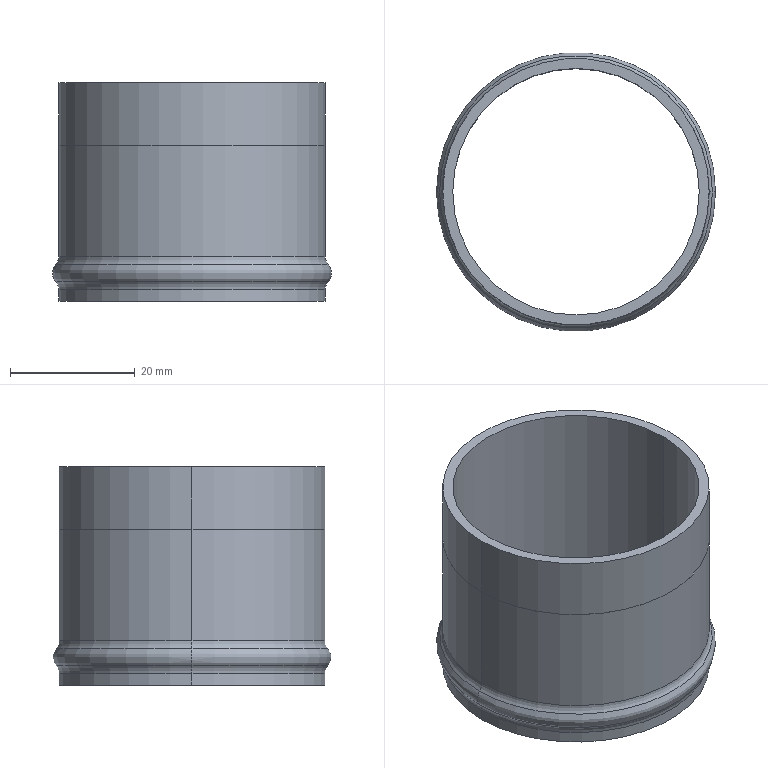Part | SolidWorks | features ICE 1, RevolutionThin 1 | 1 solid | 25 faces | box 44.7 x 44.7 x 35 mm | volume 7344 mm3 | torus 12 | cylinder 10 | plane 3 | commonest cylinder face diameters 39.5 x4 42.7 x4 42.68 x2
STEP:
#1=CARTESIAN_POINT('',(21.34,0.,-10.));
#2=VERTEX_POINT('',#1);
#3=CARTESIAN_POINT('',(-21.34,0.,-10.));
#4=VERTEX_POINT('',#3);
#5=CARTESIAN_POINT('',(0.,0.,-10.));
#6=DIRECTION('',(0.,0.,1.));
#7=DIRECTION('',(1.,0.,0.));
#8=AXIS2_PLACEMENT_3D('',#5,#6,#7);
#9=CIRCLE('',#8,21.34);
#10=EDGE_CURVE('',#2,#4,#9,.T.);
#11=ORIENTED_EDGE('',*,*,#10,.T.);
#12=CARTESIAN_POINT('',(-21.34,0.,0.));
#13=VERTEX_POINT('',#12);
#14=CARTESIAN_POINT('',(-21.34,0.,-10.));
#15=DIRECTION('',(0.,0.,1.));
#16=VECTOR('',#15,1000.);
#17=LINE('',#14,#16);
#18=EDGE_CURVE('',#4,#13,#17,.T.);
#19=ORIENTED_EDGE('',*,*,#18,.T.);
#20=CARTESIAN_POINT('',(21.34,0.,0.));
#21=VERTEX_POINT('',#20);
#22=CARTESIAN_POINT('',(0.,0.,0.));
#23=DIRECTION('',(0.,0.,1.));
#24=DIRECTION('',(1.,0.,0.));
#25=AXIS2_PLACEMENT_3D('',#22,#23,#24);
#26=CIRCLE('',#25,21.34);
#27=EDGE_CURVE('',#21,#13,#26,.T.);
#28=ORIENTED_EDGE('',*,*,#27,.F.);
#29=CARTESIAN_POINT('',(21.34,0.,-10.));
#30=DIRECTION('',(0.,0.,1.));
#31=VECTOR('',#30,1000.);
#32=LINE('',#29,#31);
#33=EDGE_CURVE('',#2,#21,#32,.T.);
#34=ORIENTED_EDGE('',*,*,#33,.F.);
#35=EDGE_LOOP('',(#11,#19,#28,#34));
#36=FACE_OUTER_BOUND('',#35,.T.);
#37=CARTESIAN_POINT('',(0.,0.,-10.));
#38=DIRECTION('',(0.,0.,1.));
#39=DIRECTION('',(1.,0.,0.));
#40=AXIS2_PLACEMENT_3D('',#37,#38,#39);
#41=CYLINDRICAL_SURFACE('',#40,21.34);
#42=ADVANCED_FACE('',(#36),#41,.T.);
#43=CARTESIAN_POINT('',(20.65,0.,-30.765));
#44=VERTEX_POINT('',#43);
#45=CARTESIAN_POINT('',(-20.65,0.,-30.765));
#46=VERTEX_POINT('',#45);
#47=CARTESIAN_POINT('',(0.,0.,-30.765));
#48=DIRECTION('',(0.,0.,1.));
#49=DIRECTION('',(1.,0.,0.));
#50=AXIS2_PLACEMENT_3D('',#47,#48,#49);
#51=CIRCLE('',#50,20.65);
#52=EDGE_CURVE('',#44,#46,#51,.T.);
#53=ORIENTED_EDGE('',*,*,#52,.T.);
#54=CARTESIAN_POINT('',(-19.75,0.,-33.146));
#55=VERTEX_POINT('',#54);
#56=CARTESIAN_POINT('',(-23.35,0.,-33.146));
#57=DIRECTION('',(0.,1.,0.));
#58=DIRECTION('',(-1.,0.,0.));
#59=AXIS2_PLACEMENT_3D('',#56,#57,#58);
#60=CIRCLE('',#59,3.6);
#61=EDGE_CURVE('',#46,#55,#60,.T.);
#62=ORIENTED_EDGE('',*,*,#61,.T.);
#63=CARTESIAN_POINT('',(19.75,0.,-33.146));
#64=VERTEX_POINT('',#63);
#65=CARTESIAN_POINT('',(0.,0.,-33.146));
#66=DIRECTION('',(0.,0.,1.));
#67=DIRECTION('',(1.,0.,0.));
#68=AXIS2_PLACEMENT_3D('',#65,#66,#67);
#69=CIRCLE('',#68,19.75);
#70=EDGE_CURVE('',#64,#55,#69,.T.);
#71=ORIENTED_EDGE('',*,*,#70,.F.);
#72=CARTESIAN_POINT('',(23.35,0.,-33.146));
#73=DIRECTION('',(0.,-1.,0.));
#74=DIRECTION('',(0.,0.,-1.));
#75=AXIS2_PLACEMENT_3D('',#72,#73,#74);
#76=CIRCLE('',#75,3.6);
#77=EDGE_CURVE('',#44,#64,#76,.T.);
#78=ORIENTED_EDGE('',*,*,#77,.F.);
#79=EDGE_LOOP('',(#53,#62,#71,#78));
#80=FACE_OUTER_BOUND('',#79,.T.);
#81=CARTESIAN_POINT('',(0.,0.,-33.146));
#82=DIRECTION('',(0.,0.,1.));
#83=DIRECTION('',(1.,0.,0.));
#84=AXIS2_PLACEMENT_3D('',#81,#82,#83);
#85=TOROIDAL_SURFACE('',#84,23.35,3.6);
#86=ADVANCED_FACE('',(#80),#85,.T.);
#87=CARTESIAN_POINT('',(0.,0.,-30.765));
#88=DIRECTION('',(0.,0.,1.));
#89=DIRECTION('',(1.,0.,0.));
#90=AXIS2_PLACEMENT_3D('',#87,#88,#89);
#91=CIRCLE('',#90,20.65);
#92=EDGE_CURVE('',#46,#44,#91,.T.);
#93=ORIENTED_EDGE('',*,*,#92,.F.);
#94=CARTESIAN_POINT('',(-20.65,0.,-30.235));
#95=VERTEX_POINT('',#94);
#96=CARTESIAN_POINT('',(-20.35,0.,-30.5));
#97=DIRECTION('',(0.,1.,0.));
#98=DIRECTION('',(-1.,0.,0.));
#99=AXIS2_PLACEMENT_3D('',#96,#97,#98);
#100=CIRCLE('',#99,0.4);
#101=EDGE_CURVE('',#46,#95,#100,.T.);
#102=ORIENTED_EDGE('',*,*,#101,.T.);
#103=CARTESIAN_POINT('',(20.65,0.,-30.235));
#104=VERTEX_POINT('',#103);
#105=CARTESIAN_POINT('',(0.,0.,-30.235));
#106=DIRECTION('',(0.,0.,1.));
#107=DIRECTION('',(1.,0.,0.));
#108=AXIS2_PLACEMENT_3D('',#105,#106,#107);
#109=CIRCLE('',#108,20.65);
#110=EDGE_CURVE('',#95,#104,#109,.T.);
#111=ORIENTED_EDGE('',*,*,#110,.T.);
#112=CARTESIAN_POINT('',(20.35,0.,-30.5));
#113=DIRECTION('',(0.,-1.,0.));
#114=DIRECTION('',(0.,0.,-1.));
#115=AXIS2_PLACEMENT_3D('',#112,#113,#114);
#116=CIRCLE('',#115,0.4);
#117=EDGE_CURVE('',#44,#104,#116,.T.);
#118=ORIENTED_EDGE('',*,*,#117,.F.);
#119=EDGE_LOOP('',(#93,#102,#111,#118));
#120=FACE_OUTER_BOUND('',#119,.T.);
#121=CARTESIAN_POINT('',(0.,0.,-30.5));
#122=DIRECTION('',(0.,0.,1.));
#123=DIRECTION('',(1.,0.,0.));
#124=AXIS2_PLACEMENT_3D('',#121,#122,#123);
#125=TOROIDAL_SURFACE('',#124,20.35,0.4);
#126=ADVANCED_FACE('',(#120),#125,.F.);
#127=CARTESIAN_POINT('',(19.75,0.,-27.854));
#128=VERTEX_POINT('',#127);
#129=CARTESIAN_POINT('',(-19.75,0.,-27.854));
#130=VERTEX_POINT('',#129);
#131=CARTESIAN_POINT('',(0.,0.,-27.854));
#132=DIRECTION('',(0.,0.,1.));
#133=DIRECTION('',(1.,0.,0.));
#134=AXIS2_PLACEMENT_3D('',#131,#132,#133);
#135=CIRCLE('',#134,19.75);
#136=EDGE_CURVE('',#128,#130,#135,.T.);
#137=ORIENTED_EDGE('',*,*,#136,.T.);
#138=CARTESIAN_POINT('',(-23.35,0.,-27.854));
#139=DIRECTION('',(0.,1.,0.));
#140=DIRECTION('',(-1.,0.,0.));
#141=AXIS2_PLACEMENT_3D('',#138,#139,#140);
#142=CIRCLE('',#141,3.6);
#143=EDGE_CURVE('',#130,#95,#142,.T.);
#144=ORIENTED_EDGE('',*,*,#143,.T.);
#145=CARTESIAN_POINT('',(0.,0.,-30.235));
#146=DIRECTION('',(0.,0.,1.));
#147=DIRECTION('',(1.,0.,0.));
#148=AXIS2_PLACEMENT_3D('',#145,#146,#147);
#149=CIRCLE('',#148,20.65);
#150=EDGE_CURVE('',#104,#95,#149,.T.);
#151=ORIENTED_EDGE('',*,*,#150,.F.);
#152=CARTESIAN_POINT('',(23.35,0.,-27.854));
#153=DIRECTION('',(0.,-1.,0.));
#154=DIRECTION('',(0.,0.,-1.));
#155=AXIS2_PLACEMENT_3D('',#152,#153,#154);
#156=CIRCLE('',#155,3.6);
#157=EDGE_CURVE('',#128,#104,#156,.T.);
#158=ORIENTED_EDGE('',*,*,#157,.F.);
#159=EDGE_LOOP('',(#137,#144,#151,#158));
#160=FACE_OUTER_BOUND('',#159,.T.);
#161=CARTESIAN_POINT('',(0.,0.,-27.854));
#162=DIRECTION('',(0.,0.,1.));
#163=DIRECTION('',(1.,0.,0.));
#164=AXIS2_PLACEMENT_3D('',#161,#162,#163);
#165=TOROIDAL_SURFACE('',#164,23.35,3.6);
#166=ADVANCED_FACE('',(#160),#165,.T.);
#167=CARTESIAN_POINT('',(0.,0.,-27.854));
#168=DIRECTION('',(0.,0.,1.));
#169=DIRECTION('',(1.,0.,0.));
#170=AXIS2_PLACEMENT_3D('',#167,#168,#169);
#171=CIRCLE('',#170,19.75);
#172=EDGE_CURVE('',#130,#128,#171,.T.);
#173=ORIENTED_EDGE('',*,*,#172,.F.);
#174=CARTESIAN_POINT('',(-19.75,0.,0.));
#175=VERTEX_POINT('',#174);
#176=CARTESIAN_POINT('',(-19.75,0.,0.));
#177=DIRECTION('',(0.,0.,1.));
#178=VECTOR('',#177,1000.);
#179=LINE('',#176,#178);
#180=EDGE_CURVE('',#130,#175,#179,.T.);
#181=ORIENTED_EDGE('',*,*,#180,.T.);
#182=CARTESIAN_POINT('',(19.75,0.,0.));
#183=VERTEX_POINT('',#182);
#184=CARTESIAN_POINT('',(0.,0.,0.));
#185=DIRECTION('',(0.,0.,1.));
#186=DIRECTION('',(1.,0.,0.));
#187=AXIS2_PLACEMENT_3D('',#184,#185,#186);
#188=CIRCLE('',#187,19.75);
#189=EDGE_CURVE('',#175,#183,#188,.T.);
#190=ORIENTED_EDGE('',*,*,#189,.T.);
#191=CARTESIAN_POINT('',(19.75,0.,0.));
#192=DIRECTION('',(0.,0.,1.));
#193=VECTOR('',#192,1000.);
#194=LINE('',#191,#193);
#195=EDGE_CURVE('',#128,#183,#194,.T.);
#196=ORIENTED_EDGE('',*,*,#195,.F.);
#197=EDGE_LOOP('',(#173,#181,#190,#196));
#198=FACE_OUTER_BOUND('',#197,.T.);
#199=CARTESIAN_POINT('',(0.,0.,0.));
#200=DIRECTION('',(0.,0.,1.));
#201=DIRECTION('',(1.,0.,0.));
#202=AXIS2_PLACEMENT_3D('',#199,#200,#201);
#203=CYLINDRICAL_SURFACE('',#202,19.75);
#204=ADVANCED_FACE('',(#198),#203,.F.);
#205=CARTESIAN_POINT('',(-21.35,0.,-27.854));
#206=VERTEX_POINT('',#205);
#207=CARTESIAN_POINT('',(21.35,0.,-27.854));
#208=VERTEX_POINT('',#207);
#209=CARTESIAN_POINT('',(0.,0.,-27.854));
#210=DIRECTION('',(0.,0.,1.));
#211=DIRECTION('',(1.,0.,0.));
#212=AXIS2_PLACEMENT_3D('',#209,#210,#211);
#213=CIRCLE('',#212,21.35);
#214=EDGE_CURVE('',#206,#208,#213,.T.);
#215=ORIENTED_EDGE('',*,*,#214,.F.);
#216=CARTESIAN_POINT('',(-21.85,0.,-29.177));
#217=VERTEX_POINT('',#216);
#218=CARTESIAN_POINT('',(-23.35,0.,-27.854));
#219=DIRECTION('',(0.,1.,0.));
#220=DIRECTION('',(-1.,0.,0.));
#221=AXIS2_PLACEMENT_3D('',#218,#219,#220);
#222=CIRCLE('',#221,2.);
#223=EDGE_CURVE('',#206,#217,#222,.T.);
#224=ORIENTED_EDGE('',*,*,#223,.T.);
#225=CARTESIAN_POINT('',(21.85,0.,-29.177));
#226=VERTEX_POINT('',#225);
#227=CARTESIAN_POINT('',(0.,0.,-29.177));
#228=DIRECTION('',(0.,0.,1.));
#229=DIRECTION('',(1.,0.,0.));
#230=AXIS2_PLACEMENT_3D('',#227,#228,#229);
#231=CIRCLE('',#230,21.85);
#232=EDGE_CURVE('',#217,#226,#231,.T.);
#233=ORIENTED_EDGE('',*,*,#232,.T.);
#234=CARTESIAN_POINT('',(23.35,0.,-27.854));
#235=DIRECTION('',(0.,-1.,0.));
#236=DIRECTION('',(0.,0.,-1.));
#237=AXIS2_PLACEMENT_3D('',#234,#235,#236);
#238=CIRCLE('',#237,2.);
#239=EDGE_CURVE('',#208,#226,#238,.T.);
#240=ORIENTED_EDGE('',*,*,#239,.F.);
#241=EDGE_LOOP('',(#215,#224,#233,#240));
#242=FACE_OUTER_BOUND('',#241,.T.);
#243=CARTESIAN_POINT('',(0.,0.,-27.854));
#244=DIRECTION('',(0.,0.,1.));
#245=DIRECTION('',(1.,0.,0.));
#246=AXIS2_PLACEMENT_3D('',#243,#244,#245);
#247=TOROIDAL_SURFACE('',#246,23.35,2.);
#248=ADVANCED_FACE('',(#242),#247,.F.);
#249=CARTESIAN_POINT('',(21.85,0.,-31.823));
#250=VERTEX_POINT('',#249);
#251=CARTESIAN_POINT('',(-21.85,0.,-31.823));
#252=VERTEX_POINT('',#251);
#253=CARTESIAN_POINT('',(0.,0.,-31.823));
#254=DIRECTION('',(0.,0.,1.));
#255=DIRECTION('',(1.,0.,0.));
#256=AXIS2_PLACEMENT_3D('',#253,#254,#255);
#257=CIRCLE('',#256,21.85);
#258=EDGE_CURVE('',#250,#252,#257,.T.);
#259=ORIENTED_EDGE('',*,*,#258,.T.);
#260=CARTESIAN_POINT('',(-20.35,0.,-30.5));
#261=DIRECTION('',(0.,1.,0.));
#262=DIRECTION('',(-1.,0.,0.));
#263=AXIS2_PLACEMENT_3D('',#260,#261,#262);
#264=CIRCLE('',#263,2.);
#265=EDGE_CURVE('',#252,#217,#264,.T.);
#266=ORIENTED_EDGE('',*,*,#265,.T.);
#267=CARTESIAN_POINT('',(0.,0.,-29.177));
#268=DIRECTION('',(0.,0.,1.));
#269=DIRECTION('',(1.,0.,0.));
#270=AXIS2_PLACEMENT_3D('',#267,#268,#269);
#271=CIRCLE('',#270,21.85);
#272=EDGE_CURVE('',#226,#217,#271,.T.);
#273=ORIENTED_EDGE('',*,*,#272,.F.);
#274=CARTESIAN_POINT('',(20.35,0.,-30.5));
#275=DIRECTION('',(0.,-1.,0.));
#276=DIRECTION('',(0.,0.,-1.));
#277=AXIS2_PLACEMENT_3D('',#274,#275,#276);
#278=CIRCLE('',#277,2.);
#279=EDGE_CURVE('',#250,#226,#278,.T.);
#280=ORIENTED_EDGE('',*,*,#279,.F.);
#281=EDGE_LOOP('',(#259,#266,#273,#280));
#282=FACE_OUTER_BOUND('',#281,.T.);
#283=CARTESIAN_POINT('',(0.,0.,-30.5));
#284=DIRECTION('',(0.,0.,1.));
#285=DIRECTION('',(1.,0.,0.));
#286=AXIS2_PLACEMENT_3D('',#283,#284,#285);
#287=TOROIDAL_SURFACE('',#286,20.35,2.);
#288=ADVANCED_FACE('',(#282),#287,.T.);
#289=CARTESIAN_POINT('',(0.,0.,-31.823));
#290=DIRECTION('',(0.,0.,1.));
#291=DIRECTION('',(1.,0.,0.));
#292=AXIS2_PLACEMENT_3D('',#289,#290,#291);
#293=CIRCLE('',#292,21.85);
#294=EDGE_CURVE('',#252,#250,#293,.T.);
#295=ORIENTED_EDGE('',*,*,#294,.F.);
#296=CARTESIAN_POINT('',(-21.35,0.,-33.146));
#297=VERTEX_POINT('',#296);
#298=CARTESIAN_POINT('',(-23.35,0.,-33.146));
#299=DIRECTION('',(0.,1.,0.));
#300=DIRECTION('',(-1.,0.,0.));
#301=AXIS2_PLACEMENT_3D('',#298,#299,#300);
#302=CIRCLE('',#301,2.);
#303=EDGE_CURVE('',#252,#297,#302,.T.);
#304=ORIENTED_EDGE('',*,*,#303,.T.);
#305=CARTESIAN_POINT('',(21.35,0.,-33.146));
#306=VERTEX_POINT('',#305);
#307=CARTESIAN_POINT('',(0.,0.,-33.146));
#308=DIRECTION('',(0.,0.,1.));
#309=DIRECTION('',(1.,0.,0.));
#310=AXIS2_PLACEMENT_3D('',#307,#308,#309);
#311=CIRCLE('',#310,21.35);
#312=EDGE_CURVE('',#297,#306,#311,.T.);
#313=ORIENTED_EDGE('',*,*,#312,.T.);
#314=CARTESIAN_POINT('',(23.35,0.,-33.146));
#315=DIRECTION('',(0.,-1.,0.));
#316=DIRECTION('',(0.,0.,-1.));
#317=AXIS2_PLACEMENT_3D('',#314,#315,#316);
#318=CIRCLE('',#317,2.);
#319=EDGE_CURVE('',#250,#306,#318,.T.);
#320=ORIENTED_EDGE('',*,*,#319,.F.);
#321=EDGE_LOOP('',(#295,#304,#313,#320));
#322=FACE_OUTER_BOUND('',#321,.T.);
#323=CARTESIAN_POINT('',(0.,0.,-33.146));
#324=DIRECTION('',(0.,0.,1.));
#325=DIRECTION('',(1.,0.,0.));
#326=AXIS2_PLACEMENT_3D('',#323,#324,#325);
#327=TOROIDAL_SURFACE('',#326,23.35,2.);
#328=ADVANCED_FACE('',(#322),#327,.F.);
#329=CARTESIAN_POINT('',(21.35,0.,-35.));
#330=VERTEX_POINT('',#329);
#331=CARTESIAN_POINT('',(-21.35,0.,-35.));
#332=VERTEX_POINT('',#331);
#333=CARTESIAN_POINT('',(0.,0.,-35.));
#334=DIRECTION('',(0.,0.,1.));
#335=DIRECTION('',(1.,0.,0.));
#336=AXIS2_PLACEMENT_3D('',#333,#334,#335);
#337=CIRCLE('',#336,21.35);
#338=EDGE_CURVE('',#330,#332,#337,.T.);
#339=ORIENTED_EDGE('',*,*,#338,.T.);
#340=CARTESIAN_POINT('',(-21.35,0.,0.));
#341=DIRECTION('',(0.,0.,1.));
#342=VECTOR('',#341,1000.);
#343=LINE('',#340,#342);
#344=EDGE_CURVE('',#332,#297,#343,.T.);
#345=ORIENTED_EDGE('',*,*,#344,.T.);
#346=CARTESIAN_POINT('',(0.,0.,-33.146));
#347=DIRECTION('',(0.,0.,1.));
#348=DIRECTION('',(1.,0.,0.));
#349=AXIS2_PLACEMENT_3D('',#346,#347,#348);
#350=CIRCLE('',#349,21.35);
#351=EDGE_CURVE('',#306,#297,#350,.T.);
#352=ORIENTED_EDGE('',*,*,#351,.F.);
#353=CARTESIAN_POINT('',(21.35,0.,0.));
#354=DIRECTION('',(0.,0.,1.));
#355=VECTOR('',#354,1000.);
#356=LINE('',#353,#355);
#357=EDGE_CURVE('',#330,#306,#356,.T.);
#358=ORIENTED_EDGE('',*,*,#357,.F.);
#359=EDGE_LOOP('',(#339,#345,#352,#358));
#360=FACE_OUTER_BOUND('',#359,.T.);
#361=CARTESIAN_POINT('',(0.,0.,0.));
#362=DIRECTION('',(0.,0.,1.));
#363=DIRECTION('',(1.,0.,0.));
#364=AXIS2_PLACEMENT_3D('',#361,#362,#363);
#365=CYLINDRICAL_SURFACE('',#364,21.35);
#366=ADVANCED_FACE('',(#360),#365,.T.);
#367=CARTESIAN_POINT('',(-19.75,0.,-35.));
#368=VERTEX_POINT('',#367);
#369=CARTESIAN_POINT('',(19.75,0.,-35.));
#370=VERTEX_POINT('',#369);
#371=CARTESIAN_POINT('',(0.,0.,-35.));
#372=DIRECTION('',(0.,0.,1.));
#373=DIRECTION('',(1.,0.,0.));
#374=AXIS2_PLACEMENT_3D('',#371,#372,#373);
#375=CIRCLE('',#374,19.75);
#376=EDGE_CURVE('',#368,#370,#375,.T.);
#377=ORIENTED_EDGE('',*,*,#376,.F.);
#378=CARTESIAN_POINT('',(-19.75,0.,0.));
#379=DIRECTION('',(0.,0.,1.));
#380=VECTOR('',#379,1000.);
#381=LINE('',#378,#380);
#382=EDGE_CURVE('',#368,#55,#381,.T.);
#383=ORIENTED_EDGE('',*,*,#382,.T.);
#384=CARTESIAN_POINT('',(0.,0.,-33.146));
#385=DIRECTION('',(0.,0.,1.));
#386=DIRECTION('',(1.,0.,0.));
#387=AXIS2_PLACEMENT_3D('',#384,#385,#386);
#388=CIRCLE('',#387,19.75);
#389=EDGE_CURVE('',#55,#64,#388,.T.);
#390=ORIENTED_EDGE('',*,*,#389,.T.);
#391=CARTESIAN_POINT('',(19.75,0.,0.));
#392=DIRECTION('',(0.,0.,1.));
#393=VECTOR('',#392,1000.);
#394=LINE('',#391,#393);
#395=EDGE_CURVE('',#370,#64,#394,.T.);
#396=ORIENTED_EDGE('',*,*,#395,.F.);
#397=EDGE_LOOP('',(#377,#383,#390,#396));
#398=FACE_OUTER_BOUND('',#397,.T.);
#399=CARTESIAN_POINT('',(0.,0.,0.));
#400=DIRECTION('',(0.,0.,1.));
#401=DIRECTION('',(1.,0.,0.));
#402=AXIS2_PLACEMENT_3D('',#399,#400,#401);
#403=CYLINDRICAL_SURFACE('',#402,19.75);
#404=ADVANCED_FACE('',(#398),#403,.F.);
#405=CARTESIAN_POINT('',(0.,0.,-27.854));
#406=DIRECTION('',(0.,0.,1.));
#407=DIRECTION('',(1.,0.,0.));
#408=AXIS2_PLACEMENT_3D('',#405,#406,#407);
#409=CIRCLE('',#408,21.35);
#410=EDGE_CURVE('',#208,#206,#409,.T.);
#411=ORIENTED_EDGE('',*,*,#410,.T.);
#412=CARTESIAN_POINT('',(-21.35,0.,-10.));
#413=VERTEX_POINT('',#412);
#414=CARTESIAN_POINT('',(-21.35,0.,0.));
#415=DIRECTION('',(0.,0.,1.));
#416=VECTOR('',#415,1000.);
#417=LINE('',#414,#416);
#418=EDGE_CURVE('',#206,#413,#417,.T.);
#419=ORIENTED_EDGE('',*,*,#418,.T.);
#420=CARTESIAN_POINT('',(21.35,0.,-10.));
#421=VERTEX_POINT('',#420);
#422=CARTESIAN_POINT('',(0.,0.,-10.));
#423=DIRECTION('',(0.,0.,1.));
#424=DIRECTION('',(1.,0.,0.));
#425=AXIS2_PLACEMENT_3D('',#422,#423,#424);
#426=CIRCLE('',#425,21.35);
#427=EDGE_CURVE('',#421,#413,#426,.T.);
#428=ORIENTED_EDGE('',*,*,#427,.F.);
#429=CARTESIAN_POINT('',(21.35,0.,0.));
#430=DIRECTION('',(0.,0.,1.));
#431=VECTOR('',#430,1000.);
#432=LINE('',#429,#431);
#433=EDGE_CURVE('',#208,#421,#432,.T.);
#434=ORIENTED_EDGE('',*,*,#433,.F.);
#435=EDGE_LOOP('',(#411,#419,#428,#434));
#436=FACE_OUTER_BOUND('',#435,.T.);
#437=CARTESIAN_POINT('',(0.,0.,0.));
#438=DIRECTION('',(0.,0.,1.));
#439=DIRECTION('',(1.,0.,0.));
#440=AXIS2_PLACEMENT_3D('',#437,#438,#439);
#441=CYLINDRICAL_SURFACE('',#440,21.35);
#442=ADVANCED_FACE('',(#436),#441,.T.);
#443=ORIENTED_EDGE('',*,*,#418,.F.);
#444=ORIENTED_EDGE('',*,*,#214,.T.);
#445=ORIENTED_EDGE('',*,*,#433,.T.);
#446=CARTESIAN_POINT('',(0.,0.,-10.));
#447=DIRECTION('',(0.,0.,1.));
#448=DIRECTION('',(1.,0.,0.));
#449=AXIS2_PLACEMENT_3D('',#446,#447,#448);
#450=CIRCLE('',#449,21.35);
#451=EDGE_CURVE('',#413,#421,#450,.T.);
#452=ORIENTED_EDGE('',*,*,#451,.F.);
#453=EDGE_LOOP('',(#443,#444,#445,#452));
#454=FACE_OUTER_BOUND('',#453,.T.);
#455=CARTESIAN_POINT('',(0.,0.,0.));
#456=DIRECTION('',(0.,0.,1.));
#457=DIRECTION('',(1.,0.,0.));
#458=AXIS2_PLACEMENT_3D('',#455,#456,#457);
#459=CYLINDRICAL_SURFACE('',#458,21.35);
#460=ADVANCED_FACE('',(#454),#459,.T.);
#461=CARTESIAN_POINT('',(0.,0.,0.));
#462=DIRECTION('',(0.,0.,1.));
#463=DIRECTION('',(1.,0.,0.));
#464=AXIS2_PLACEMENT_3D('',#461,#462,#463);
#465=CIRCLE('',#464,19.75);
#466=EDGE_CURVE('',#183,#175,#465,.T.);
#467=ORIENTED_EDGE('',*,*,#466,.F.);
#468=ORIENTED_EDGE('',*,*,#189,.F.);
#469=EDGE_LOOP('',(#467,#468));
#470=FACE_BOUND('',#469,.T.);
#471=ORIENTED_EDGE('',*,*,#27,.T.);
#472=CARTESIAN_POINT('',(0.,0.,0.));
#473=DIRECTION('',(0.,0.,1.));
#474=DIRECTION('',(1.,0.,0.));
#475=AXIS2_PLACEMENT_3D('',#472,#473,#474);
#476=CIRCLE('',#475,21.34);
#477=EDGE_CURVE('',#13,#21,#476,.T.);
#478=ORIENTED_EDGE('',*,*,#477,.T.);
#479=EDGE_LOOP('',(#471,#478));
#480=FACE_OUTER_BOUND('',#479,.T.);
#481=CARTESIAN_POINT('',(0.,19.75,0.));
#482=DIRECTION('',(0.,0.,1.));
#483=DIRECTION('',(1.,0.,0.));
#484=AXIS2_PLACEMENT_3D('',#481,#482,#483);
#485=PLANE('',#484);
#486=ADVANCED_FACE('',(#470,#480),#485,.T.);
#487=ORIENTED_EDGE('',*,*,#382,.F.);
#488=CARTESIAN_POINT('',(0.,0.,-35.));
#489=DIRECTION('',(0.,0.,1.));
#490=DIRECTION('',(1.,0.,0.));
#491=AXIS2_PLACEMENT_3D('',#488,#489,#490);
#492=CIRCLE('',#491,19.75);
#493=EDGE_CURVE('',#370,#368,#492,.T.);
#494=ORIENTED_EDGE('',*,*,#493,.F.);
#495=ORIENTED_EDGE('',*,*,#395,.T.);
#496=ORIENTED_EDGE('',*,*,#70,.T.);
#497=EDGE_LOOP('',(#487,#494,#495,#496));
#498=FACE_OUTER_BOUND('',#497,.T.);
#499=CARTESIAN_POINT('',(0.,0.,0.));
#500=DIRECTION('',(0.,0.,1.));
#501=DIRECTION('',(1.,0.,0.));
#502=AXIS2_PLACEMENT_3D('',#499,#500,#501);
#503=CYLINDRICAL_SURFACE('',#502,19.75);
#504=ADVANCED_FACE('',(#498),#503,.F.);
#505=ORIENTED_EDGE('',*,*,#493,.T.);
#506=ORIENTED_EDGE('',*,*,#376,.T.);
#507=EDGE_LOOP('',(#505,#506));
#508=FACE_BOUND('',#507,.T.);
#509=ORIENTED_EDGE('',*,*,#338,.F.);
#510=CARTESIAN_POINT('',(0.,0.,-35.));
#511=DIRECTION('',(0.,0.,1.));
#512=DIRECTION('',(1.,0.,0.));
#513=AXIS2_PLACEMENT_3D('',#510,#511,#512);
#514=CIRCLE('',#513,21.35);
#515=EDGE_CURVE('',#332,#330,#514,.T.);
#516=ORIENTED_EDGE('',*,*,#515,.F.);
#517=EDGE_LOOP('',(#509,#516));
#518=FACE_OUTER_BOUND('',#517,.T.);
#519=CARTESIAN_POINT('',(0.,21.35,-35.));
#520=DIRECTION('',(0.,0.,-1.));
#521=DIRECTION('',(-1.,0.,0.));
#522=AXIS2_PLACEMENT_3D('',#519,#520,#521);
#523=PLANE('',#522);
#524=ADVANCED_FACE('',(#508,#518),#523,.T.);
#525=ORIENTED_EDGE('',*,*,#344,.F.);
#526=ORIENTED_EDGE('',*,*,#515,.T.);
#527=ORIENTED_EDGE('',*,*,#357,.T.);
#528=ORIENTED_EDGE('',*,*,#312,.F.);
#529=EDGE_LOOP('',(#525,#526,#527,#528));
#530=FACE_OUTER_BOUND('',#529,.T.);
#531=CARTESIAN_POINT('',(0.,0.,0.));
#532=DIRECTION('',(0.,0.,1.));
#533=DIRECTION('',(1.,0.,0.));
#534=AXIS2_PLACEMENT_3D('',#531,#532,#533);
#535=CYLINDRICAL_SURFACE('',#534,21.35);
#536=ADVANCED_FACE('',(#530),#535,.T.);
#537=ORIENTED_EDGE('',*,*,#303,.F.);
#538=ORIENTED_EDGE('',*,*,#258,.F.);
#539=ORIENTED_EDGE('',*,*,#319,.T.);
#540=ORIENTED_EDGE('',*,*,#351,.T.);
#541=EDGE_LOOP('',(#537,#538,#539,#540));
#542=FACE_OUTER_BOUND('',#541,.T.);
#543=CARTESIAN_POINT('',(0.,0.,-33.146));
#544=DIRECTION('',(0.,0.,1.));
#545=DIRECTION('',(1.,0.,0.));
#546=AXIS2_PLACEMENT_3D('',#543,#544,#545);
#547=TOROIDAL_SURFACE('',#546,23.35,2.);
#548=ADVANCED_FACE('',(#542),#547,.F.);
#549=ORIENTED_EDGE('',*,*,#265,.F.);
#550=ORIENTED_EDGE('',*,*,#294,.T.);
#551=ORIENTED_EDGE('',*,*,#279,.T.);
#552=ORIENTED_EDGE('',*,*,#232,.F.);
#553=EDGE_LOOP('',(#549,#550,#551,#552));
#554=FACE_OUTER_BOUND('',#553,.T.);
#555=CARTESIAN_POINT('',(0.,0.,-30.5));
#556=DIRECTION('',(0.,0.,1.));
#557=DIRECTION('',(1.,0.,0.));
#558=AXIS2_PLACEMENT_3D('',#555,#556,#557);
#559=TOROIDAL_SURFACE('',#558,20.35,2.);
#560=ADVANCED_FACE('',(#554),#559,.T.);
#561=ORIENTED_EDGE('',*,*,#223,.F.);
#562=ORIENTED_EDGE('',*,*,#410,.F.);
#563=ORIENTED_EDGE('',*,*,#239,.T.);
#564=ORIENTED_EDGE('',*,*,#272,.T.);
#565=EDGE_LOOP('',(#561,#562,#563,#564));
#566=FACE_OUTER_BOUND('',#565,.T.);
#567=CARTESIAN_POINT('',(0.,0.,-27.854));
#568=DIRECTION('',(0.,0.,1.));
#569=DIRECTION('',(1.,0.,0.));
#570=AXIS2_PLACEMENT_3D('',#567,#568,#569);
#571=TOROIDAL_SURFACE('',#570,23.35,2.);
#572=ADVANCED_FACE('',(#566),#571,.F.);
#573=ORIENTED_EDGE('',*,*,#180,.F.);
#574=ORIENTED_EDGE('',*,*,#136,.F.);
#575=ORIENTED_EDGE('',*,*,#195,.T.);
#576=ORIENTED_EDGE('',*,*,#466,.T.);
#577=EDGE_LOOP('',(#573,#574,#575,#576));
#578=FACE_OUTER_BOUND('',#577,.T.);
#579=CARTESIAN_POINT('',(0.,0.,0.));
#580=DIRECTION('',(0.,0.,1.));
#581=DIRECTION('',(1.,0.,0.));
#582=AXIS2_PLACEMENT_3D('',#579,#580,#581);
#583=CYLINDRICAL_SURFACE('',#582,19.75);
#584=ADVANCED_FACE('',(#578),#583,.F.);
#585=ORIENTED_EDGE('',*,*,#143,.F.);
#586=ORIENTED_EDGE('',*,*,#172,.T.);
#587=ORIENTED_EDGE('',*,*,#157,.T.);
#588=ORIENTED_EDGE('',*,*,#110,.F.);
#589=EDGE_LOOP('',(#585,#586,#587,#588));
#590=FACE_OUTER_BOUND('',#589,.T.);
#591=CARTESIAN_POINT('',(0.,0.,-27.854));
#592=DIRECTION('',(0.,0.,1.));
#593=DIRECTION('',(1.,0.,0.));
#594=AXIS2_PLACEMENT_3D('',#591,#592,#593);
#595=TOROIDAL_SURFACE('',#594,23.35,3.6);
#596=ADVANCED_FACE('',(#590),#595,.T.);
#597=ORIENTED_EDGE('',*,*,#101,.F.);
#598=ORIENTED_EDGE('',*,*,#52,.F.);
#599=ORIENTED_EDGE('',*,*,#117,.T.);
#600=ORIENTED_EDGE('',*,*,#150,.T.);
#601=EDGE_LOOP('',(#597,#598,#599,#600));
#602=FACE_OUTER_BOUND('',#601,.T.);
#603=CARTESIAN_POINT('',(0.,0.,-30.5));
#604=DIRECTION('',(0.,0.,1.));
#605=DIRECTION('',(1.,0.,0.));
#606=AXIS2_PLACEMENT_3D('',#603,#604,#605);
#607=TOROIDAL_SURFACE('',#606,20.35,0.4);
#608=ADVANCED_FACE('',(#602),#607,.F.);
#609=ORIENTED_EDGE('',*,*,#61,.F.);
#610=ORIENTED_EDGE('',*,*,#92,.T.);
#611=ORIENTED_EDGE('',*,*,#77,.T.);
#612=ORIENTED_EDGE('',*,*,#389,.F.);
#613=EDGE_LOOP('',(#609,#610,#611,#612));
#614=FACE_OUTER_BOUND('',#613,.T.);
#615=CARTESIAN_POINT('',(0.,0.,-33.146));
#616=DIRECTION('',(0.,0.,1.));
#617=DIRECTION('',(1.,0.,0.));
#618=AXIS2_PLACEMENT_3D('',#615,#616,#617);
#619=TOROIDAL_SURFACE('',#618,23.35,3.6);
#620=ADVANCED_FACE('',(#614),#619,.T.);
#621=ORIENTED_EDGE('',*,*,#10,.F.);
#622=CARTESIAN_POINT('',(0.,0.,-10.));
#623=DIRECTION('',(0.,0.,1.));
#624=DIRECTION('',(1.,0.,0.));
#625=AXIS2_PLACEMENT_3D('',#622,#623,#624);
#626=CIRCLE('',#625,21.34);
#627=EDGE_CURVE('',#4,#2,#626,.T.);
#628=ORIENTED_EDGE('',*,*,#627,.F.);
#629=EDGE_LOOP('',(#621,#628));
#630=FACE_BOUND('',#629,.T.);
#631=ORIENTED_EDGE('',*,*,#427,.T.);
#632=ORIENTED_EDGE('',*,*,#451,.T.);
#633=EDGE_LOOP('',(#631,#632));
#634=FACE_OUTER_BOUND('',#633,.T.);
#635=CARTESIAN_POINT('',(0.,0.,-10.));
#636=DIRECTION('',(0.,0.,1.));
#637=DIRECTION('',(1.,0.,0.));
#638=AXIS2_PLACEMENT_3D('',#635,#636,#637);
#639=PLANE('',#638);
#640=ADVANCED_FACE('',(#630,#634),#639,.T.);
#641=ORIENTED_EDGE('',*,*,#18,.F.);
#642=ORIENTED_EDGE('',*,*,#627,.T.);
#643=ORIENTED_EDGE('',*,*,#33,.T.);
#644=ORIENTED_EDGE('',*,*,#477,.F.);
#645=EDGE_LOOP('',(#641,#642,#643,#644));
#646=FACE_OUTER_BOUND('',#645,.T.);
#647=CARTESIAN_POINT('',(0.,0.,-10.));
#648=DIRECTION('',(0.,0.,1.));
#649=DIRECTION('',(1.,0.,0.));
#650=AXIS2_PLACEMENT_3D('',#647,#648,#649);
#651=CYLINDRICAL_SURFACE('',#650,21.34);
#652=ADVANCED_FACE('',(#646),#651,.T.);
#653=CLOSED_SHELL('',(#42,#86,#126,#166,#204,#248,#288,#328,#366,#404,#442,#460,#486,#504,#524,#536,#548,#560,#572,#584,#596,#608,#620,#640,#652));
#654=MANIFOLD_SOLID_BREP('',#653);
#655=CARTESIAN_POINT('',(0.,0.,0.));
#656=DIRECTION('',(0.,0.,1.));
#657=DIRECTION('',(1.,0.,0.));
#658=AXIS2_PLACEMENT_3D('',#655,#656,#657);
#659=(LENGTH_UNIT()NAMED_UNIT(*)SI_UNIT(.MILLI.,.METRE.));
#660=UNCERTAINTY_MEASURE_WITH_UNIT(LENGTH_MEASURE(0.00001),#659,'','');
#661=(NAMED_UNIT(*)PLANE_ANGLE_UNIT()SI_UNIT($,.RADIAN.));
#662=(NAMED_UNIT(*)SI_UNIT($,.STERADIAN.)SOLID_ANGLE_UNIT());
#663=(GEOMETRIC_REPRESENTATION_CONTEXT(3)GLOBAL_UNCERTAINTY_ASSIGNED_CONTEXT((#660))GLOBAL_UNIT_ASSIGNED_CONTEXT((#659,#661,#662))REPRESENTATION_CONTEXT('',''));
#664=ADVANCED_BREP_SHAPE_REPRESENTATION('',(#654,#658),#663);